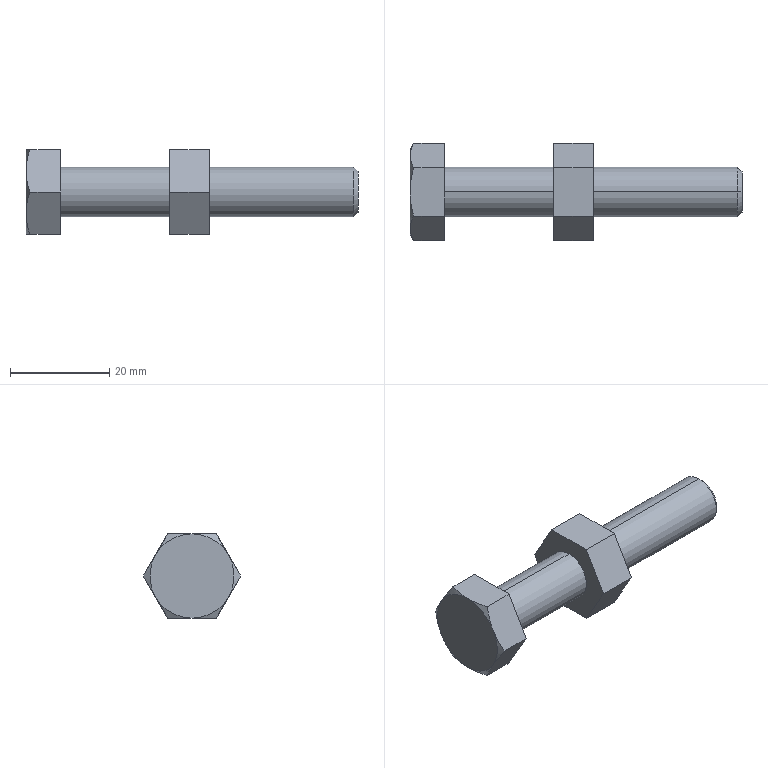Part | STEP file | M10-60_RCB10-70 | 1 solid | 29 faces | box 67 x 19.63 x 17 mm | volume 7820 mm3 | plane 17 | cone 8 | cylinder 4 | commonest cylinder face diameters 10 x4